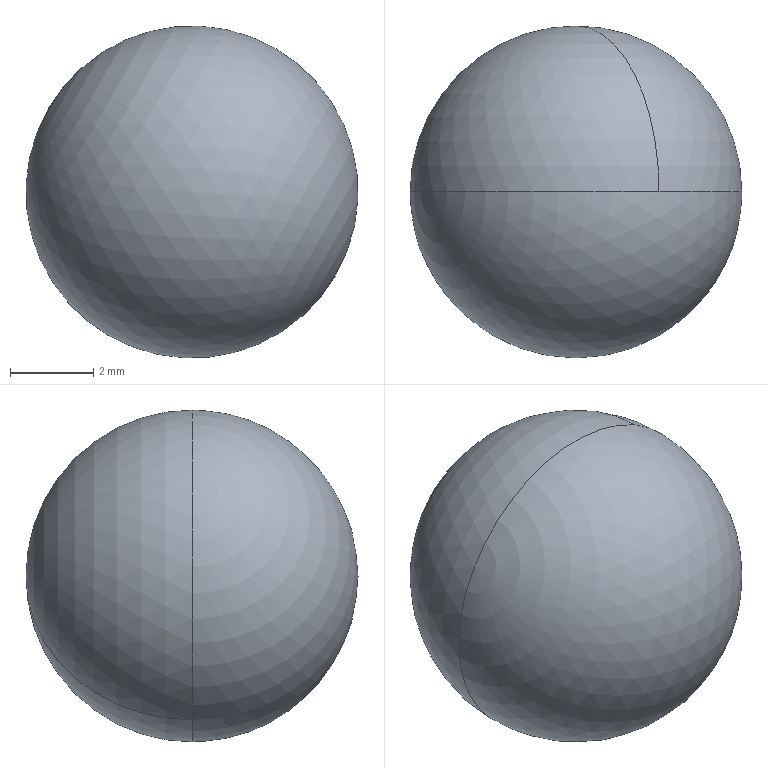Part | NX | features solid 2 | 1 solid | 3 faces | box 8 x 8 x 8 mm | volume 268.083 mm3 | sphere 3
STEP:
#1=CARTESIAN_POINT('',(212.249,-15.,-946.464));
#2=VERTEX_POINT('',#1);
#3=CARTESIAN_POINT('',(210.785,-15.,-941.));
#4=VERTEX_POINT('',#3);
#5=CARTESIAN_POINT('',(214.249,-15.,-943.));
#6=DIRECTION('',(0.,1.,0.));
#7=DIRECTION('',(-0.5,0.,-0.866));
#8=AXIS2_PLACEMENT_3D('',#5,#6,#7);
#9=CIRCLE('',#8,4.);
#10=EDGE_CURVE('',#2,#4,#9,.T.);
#11=ORIENTED_EDGE('',*,*,#10,.F.);
#12=CARTESIAN_POINT('',(217.713,-15.,-945.));
#13=VERTEX_POINT('',#12);
#14=CARTESIAN_POINT('',(214.249,-15.,-943.));
#15=DIRECTION('',(0.,1.,0.));
#16=DIRECTION('',(0.866,0.,-0.5));
#17=AXIS2_PLACEMENT_3D('',#14,#15,#16);
#18=CIRCLE('',#17,4.);
#19=EDGE_CURVE('',#13,#2,#18,.T.);
#20=ORIENTED_EDGE('',*,*,#19,.F.);
#21=CARTESIAN_POINT('',(216.249,-15.,-939.536));
#22=VERTEX_POINT('',#21);
#23=CARTESIAN_POINT('',(214.249,-15.,-943.));
#24=DIRECTION('',(0.,-1.,0.));
#25=DIRECTION('',(0.866,0.,-0.5));
#26=AXIS2_PLACEMENT_3D('',#23,#24,#25);
#27=CIRCLE('',#26,4.);
#28=EDGE_CURVE('',#22,#13,#27,.F.);
#29=ORIENTED_EDGE('',*,*,#28,.F.);
#30=CARTESIAN_POINT('',(214.249,-15.,-943.));
#31=DIRECTION('',(0.,-1.,0.));
#32=DIRECTION('',(0.5,0.,0.866));
#33=AXIS2_PLACEMENT_3D('',#30,#31,#32);
#34=CIRCLE('',#33,4.);
#35=EDGE_CURVE('',#4,#22,#34,.F.);
#36=ORIENTED_EDGE('',*,*,#35,.F.);
#37=EDGE_LOOP('',(#11,#20,#29,#36));
#38=FACE_BOUND('',#37,.T.);
#39=CARTESIAN_POINT('',(214.249,-15.,-943.));
#40=DIRECTION('',(0.866,0.,-0.5));
#41=DIRECTION('',(0.5,0.,0.866));
#42=AXIS2_PLACEMENT_3D('',#39,#40,#41);
#43=SPHERICAL_SURFACE('',#42,4.);
#44=ADVANCED_FACE('',(#38),#43,.T.);
#45=ORIENTED_EDGE('',*,*,#35,.T.);
#46=CARTESIAN_POINT('',(214.249,-11.,-943.));
#47=VERTEX_POINT('',#46);
#48=CARTESIAN_POINT('',(214.249,-15.,-943.));
#49=DIRECTION('',(-0.866,0.,0.5));
#50=DIRECTION('',(0.5,0.,0.866));
#51=AXIS2_PLACEMENT_3D('',#48,#49,#50);
#52=CIRCLE('',#51,4.);
#53=EDGE_CURVE('',#22,#47,#52,.T.);
#54=ORIENTED_EDGE('',*,*,#53,.T.);
#55=CARTESIAN_POINT('',(214.249,-15.,-943.));
#56=DIRECTION('',(0.866,0.,-0.5));
#57=DIRECTION('',(-0.5,0.,-0.866));
#58=AXIS2_PLACEMENT_3D('',#55,#56,#57);
#59=CIRCLE('',#58,4.);
#60=EDGE_CURVE('',#47,#2,#59,.F.);
#61=ORIENTED_EDGE('',*,*,#60,.T.);
#62=ORIENTED_EDGE('',*,*,#10,.T.);
#63=EDGE_LOOP('',(#45,#54,#61,#62));
#64=FACE_BOUND('',#63,.T.);
#65=CARTESIAN_POINT('',(214.249,-15.,-943.));
#66=DIRECTION('',(0.,-1.,0.));
#67=DIRECTION('',(-0.5,0.,-0.866));
#68=AXIS2_PLACEMENT_3D('',#65,#66,#67);
#69=SPHERICAL_SURFACE('',#68,4.);
#70=ADVANCED_FACE('',(#64),#69,.T.);
#71=ORIENTED_EDGE('',*,*,#19,.T.);
#72=ORIENTED_EDGE('',*,*,#60,.F.);
#73=ORIENTED_EDGE('',*,*,#53,.F.);
#74=ORIENTED_EDGE('',*,*,#28,.T.);
#75=EDGE_LOOP('',(#71,#72,#73,#74));
#76=FACE_BOUND('',#75,.T.);
#77=CARTESIAN_POINT('',(214.249,-15.,-943.));
#78=DIRECTION('',(0.,-1.,0.));
#79=DIRECTION('',(-0.5,0.,-0.866));
#80=AXIS2_PLACEMENT_3D('',#77,#78,#79);
#81=SPHERICAL_SURFACE('',#80,4.);
#82=ADVANCED_FACE('',(#76),#81,.T.);
#83=CLOSED_SHELL('',(#44,#70,#82));
#84=MANIFOLD_SOLID_BREP('',#83);
#85=(LENGTH_UNIT()NAMED_UNIT(*)SI_UNIT(.MILLI.,.METRE.));
#86=UNCERTAINTY_MEASURE_WITH_UNIT(LENGTH_MEASURE(0.00001),#85,'','');
#87=(NAMED_UNIT(*)PLANE_ANGLE_UNIT()SI_UNIT($,.RADIAN.));
#88=(NAMED_UNIT(*)SI_UNIT($,.STERADIAN.)SOLID_ANGLE_UNIT());
#89=(GEOMETRIC_REPRESENTATION_CONTEXT(3)GLOBAL_UNCERTAINTY_ASSIGNED_CONTEXT((#86))GLOBAL_UNIT_ASSIGNED_CONTEXT((#85,#87,#88))REPRESENTATION_CONTEXT('',''));
#90=ADVANCED_BREP_SHAPE_REPRESENTATION('',(#84),#89);